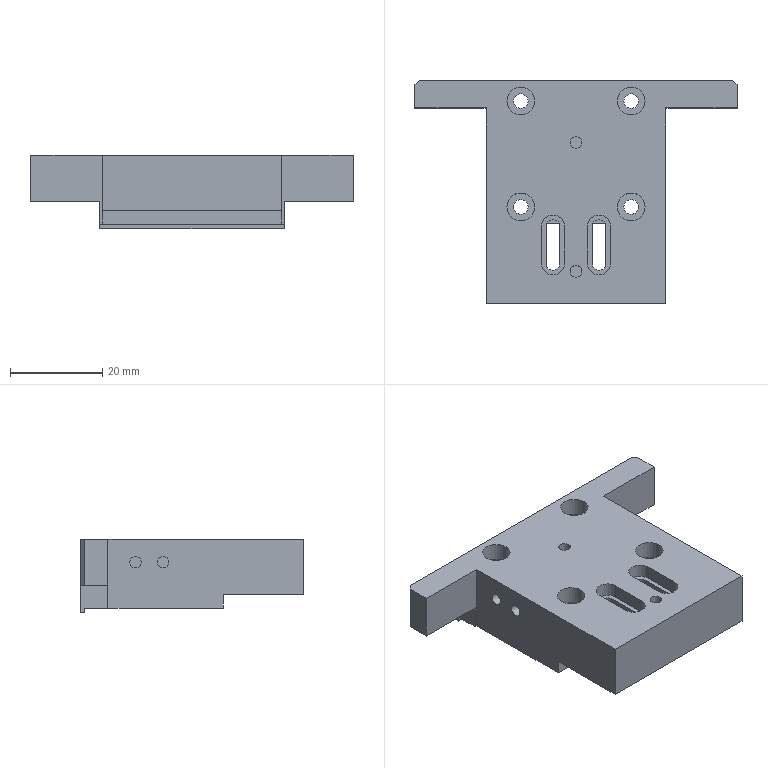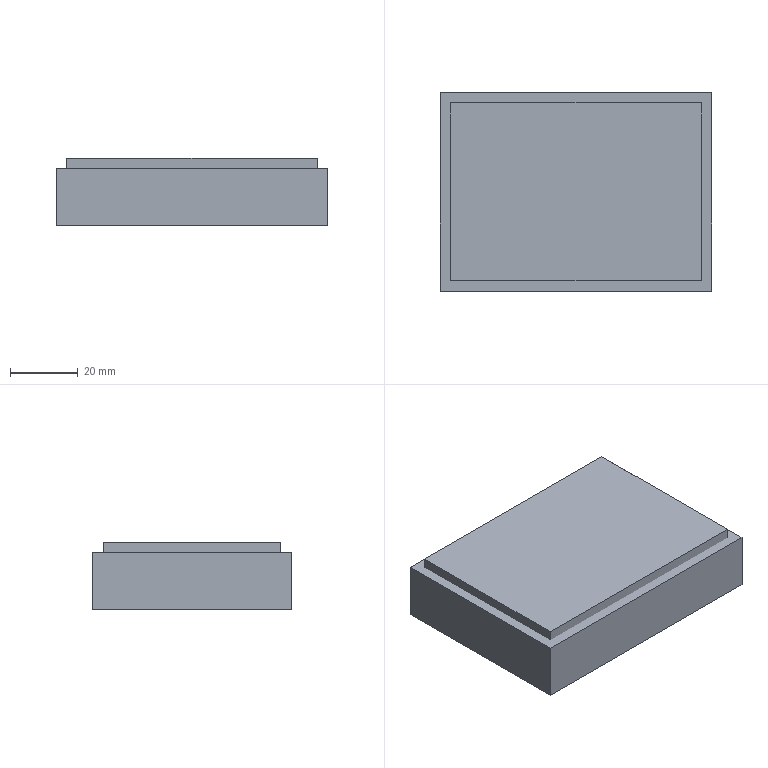CAM job | NX | 3-axis milling, drilling | part box 70 x 48.5 x 16 mm | stock box 80 x 58.5 x 20 mm
Tools:
number,name,description,diameter,corner_radius,flute_length,length,flutes
19,D80,Milling Tool-5 Parameters,80.0,0.0,50.0,75.0,2
15,D10,Milling Tool-5 Parameters,10.0,0.0,50.0,75.0,2
14,D10JING,Milling Tool-5 Parameters,10.0,0.0,50.0,75.0,2
1,D6A45,Milling Tool-5 Parameters,6.0,0.0,50.0,75.0,2
2,2.5ZT,Drilling Tool,2.5,0.0,35.0,50.0,2
16,3.2ZT,Drilling Tool,3.2,0.0,35.0,50.0,2
11,D4,Milling Tool-5 Parameters,4.0,0.0,50.0,75.0,2
17,D2,Milling Tool-5 Parameters,2.0,0.0,50.0,75.0,2
Operations:
program,operation,operation_type,tool,method,geometry_group,spindle_rpm,surface_speed,feed_per_tooth,feed_cut,feed_plunge,cut_length_mm,path_length_mm,cut_time_min,machine_time_min
1,FLOOR_WALL,VolumeBased25DMillingOperation,D80,METHOD,A,6500.0,1633.0,0.1154,1500.0,100.0,172.0,226.0,0.1147,0.1201
1,ADAPTIVE_MILLING,CavityMilling,D10,METHOD,A,9500.0,298.0,0.1579,3000.0,1000.0,4431.015,4517.015,1.479,1.488
1,ZLEVEL_PROFILE_COPY_1_COPY,ZLevelMilling,D10JING,METHOD,A,9500.0,298.0,0.0632,1200.0,1000.0,270.944,358.944,0.2267,0.2355
1,DRILLING,Operation,D6A45,METHOD,A,5000.0,94.0,0.035,350.0,0.0,24.0,214.152,0.0686,0.0876
1,DRILLING_COPY_1,Operation,2.5ZT,METHOD,A,2000.0,20.0,0.05,200.0,0.0,22.502,136.165,0.1125,0.1239
1,DRILLING_COPY_1_COPY,Operation,3.2ZT,METHOD,A,2000.0,20.0,0.05,200.0,0.0,81.846,303.267,0.4092,0.4314
1,HOLE_MILLING,CylinderMilling,D4,METHOD,A,9500.0,119.0,0.0658,1250.0,100.0,321.015,645.015,0.2568,0.2892
1,ZLEVEL_PROFILE,ZLevelMilling,D4,METHOD,A,9500.0,119.0,0.0868,1650.0,100.0,462.521,595.035,0.2803,0.2936
1,ZLEVEL_PROFILE_COPY,ZLevelMilling,D2,METHOD,A,9500.0,59.0,0.0579,1100.0,100.0,2357.546,2513.274,2.143,2.159
1,PLANAR_MILL_COPY_COPY_COPY,PlanarMilling,D6A45,METHOD,A,9500.0,179.0,0.0658,1250.0,100.0,393.749,1049.336,0.315,0.3806
2,FLOOR_WALL_COPY,VolumeBased25DMillingOperation,D80,METHOD,B,6500.0,1633.0,0.1154,1500.0,100.0,664.0,1348.001,0.4427,0.5111
2,FLOOR_WALL_1,VolumeBased25DMillingOperation,D10,METHOD,B,9500.0,298.0,0.1579,3000.0,1000.0,910.5,972.3,0.3075,0.3137
2,FLOOR_WALL_1_COPY,VolumeBased25DMillingOperation,D10,METHOD,B,9500.0,298.0,0.1579,3000.0,1000.0,1516.424,1572.224,0.5095,0.5151
2,FLOOR_WALL_1_COPY_COPY,VolumeBased25DMillingOperation,D10,METHOD,B,9500.0,298.0,0.1579,3000.0,1000.0,525.241,723.442,0.1839,0.2037
2,FLOOR_WALL_1_COPY_1,VolumeBased25DMillingOperation,D10JING,METHOD,B,9500.0,298.0,0.0789,1500.0,1000.0,676.238,1484.695,0.4677,0.5485
2,PLANAR_MILL_COPY_COPY_COPY_COPY,PlanarMilling,D6A45,METHOD,B,9500.0,179.0,0.0658,1250.0,100.0,91.493,150.093,0.0732,0.0791
2,PLANAR_MILL_COPY_COPY_COPY_COPY_COPY,PlanarMilling,D6A45,METHOD,B,9500.0,179.0,0.0658,1250.0,100.0,157.285,560.587,0.1258,0.1662
2,PLANAR_MILL_COPY_COPY_COPY_COPY_COPY_COPY,PlanarMilling,D6A45,METHOD,B,9500.0,179.0,0.0658,1250.0,100.0,118.328,345.314,0.0947,0.1174
2,PLANAR_MILL_COPY_COPY_COPY_COPY_COPY_COPY_COPY,PlanarMilling,D6A45,METHOD,B,9500.0,179.0,0.0658,1250.0,100.0,89.893,435.364,0.0719,0.1065